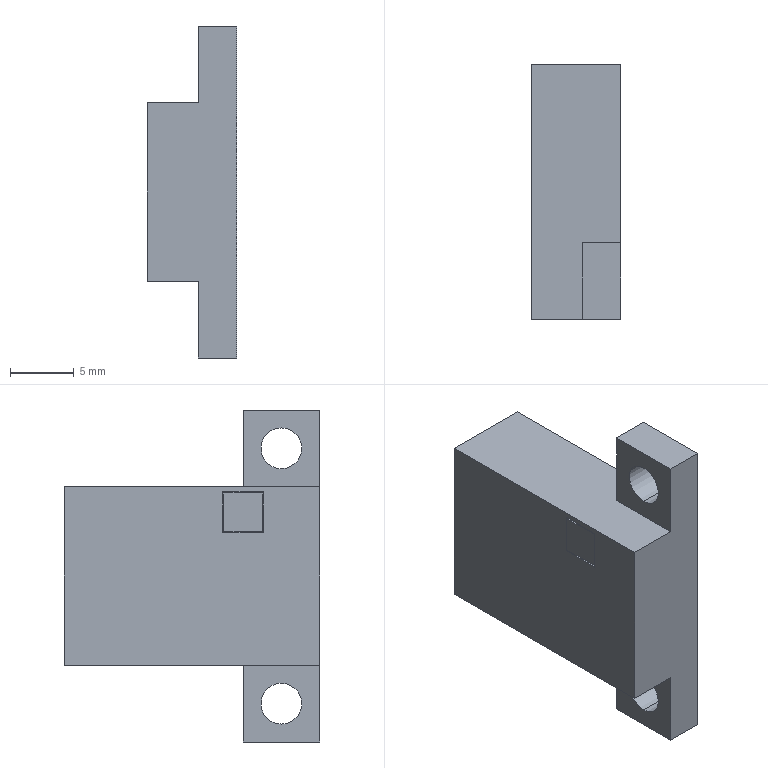Part | STEP file | 0243_104_Sensor_EE-SPY402 | 1 solid | 26 faces | box 7 x 20 x 26 mm | volume 2123 mm3 | plane 22 | cylinder 4 | commonest cylinder face diameters 3.2 x4